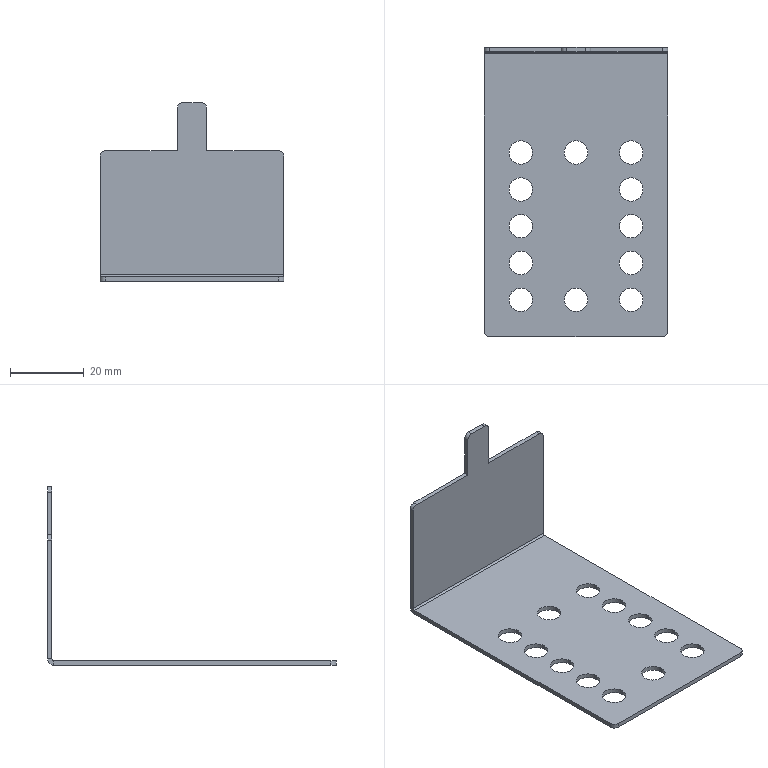Part | SolidWorks | features ICE 2, Extrusion 1, Fillet 1, FlatPattern 1, SheetMetal 1, SolidToSheetMetal 1 | 1 solid | 48 faces | box 50 x 78.5 x 48.5 mm | volume 6398 mm3 | cylinder 32 | plane 16 | commonest cylinder face diameters 6.4 x24 3 x6 1 x1 3.4 x1
STEP:
#1=CARTESIAN_POINT('',(-18.2,10.,0.));
#2=VERTEX_POINT('',#1);
#3=CARTESIAN_POINT('',(-11.8,10.,0.));
#4=VERTEX_POINT('',#3);
#5=CARTESIAN_POINT('',(-15.,10.,0.));
#6=DIRECTION('',(0.,0.,1.));
#7=DIRECTION('',(1.,0.,0.));
#8=AXIS2_PLACEMENT_3D('',#5,#6,#7);
#9=CIRCLE('',#8,3.2);
#10=EDGE_CURVE('',#2,#4,#9,.T.);
#11=ORIENTED_EDGE('',*,*,#10,.F.);
#12=CARTESIAN_POINT('',(-18.2,10.,1.2));
#13=VERTEX_POINT('',#12);
#14=CARTESIAN_POINT('',(-18.2,10.,0.));
#15=DIRECTION('',(0.,0.,1.));
#16=VECTOR('',#15,1000.);
#17=LINE('',#14,#16);
#18=EDGE_CURVE('',#2,#13,#17,.T.);
#19=ORIENTED_EDGE('',*,*,#18,.T.);
#20=CARTESIAN_POINT('',(-11.8,10.,1.2));
#21=VERTEX_POINT('',#20);
#22=CARTESIAN_POINT('',(-15.,10.,1.2));
#23=DIRECTION('',(0.,0.,1.));
#24=DIRECTION('',(1.,0.,0.));
#25=AXIS2_PLACEMENT_3D('',#22,#23,#24);
#26=CIRCLE('',#25,3.2);
#27=EDGE_CURVE('',#13,#21,#26,.T.);
#28=ORIENTED_EDGE('',*,*,#27,.T.);
#29=CARTESIAN_POINT('',(-11.8,10.,0.));
#30=DIRECTION('',(0.,0.,1.));
#31=VECTOR('',#30,1000.);
#32=LINE('',#29,#31);
#33=EDGE_CURVE('',#4,#21,#32,.T.);
#34=ORIENTED_EDGE('',*,*,#33,.F.);
#35=EDGE_LOOP('',(#11,#19,#28,#34));
#36=FACE_OUTER_BOUND('',#35,.T.);
#37=CARTESIAN_POINT('',(-15.,10.,0.));
#38=DIRECTION('',(0.,0.,1.));
#39=DIRECTION('',(1.,0.,0.));
#40=AXIS2_PLACEMENT_3D('',#37,#38,#39);
#41=CYLINDRICAL_SURFACE('',#40,3.2);
#42=ADVANCED_FACE('',(#36),#41,.F.);
#43=CARTESIAN_POINT('',(-18.2,40.,0.));
#44=VERTEX_POINT('',#43);
#45=CARTESIAN_POINT('',(-11.8,40.,0.));
#46=VERTEX_POINT('',#45);
#47=CARTESIAN_POINT('',(-15.,40.,0.));
#48=DIRECTION('',(0.,0.,1.));
#49=DIRECTION('',(1.,0.,0.));
#50=AXIS2_PLACEMENT_3D('',#47,#48,#49);
#51=CIRCLE('',#50,3.2);
#52=EDGE_CURVE('',#44,#46,#51,.T.);
#53=ORIENTED_EDGE('',*,*,#52,.F.);
#54=CARTESIAN_POINT('',(-18.2,40.,1.2));
#55=VERTEX_POINT('',#54);
#56=CARTESIAN_POINT('',(-18.2,40.,0.));
#57=DIRECTION('',(0.,0.,1.));
#58=VECTOR('',#57,1000.);
#59=LINE('',#56,#58);
#60=EDGE_CURVE('',#44,#55,#59,.T.);
#61=ORIENTED_EDGE('',*,*,#60,.T.);
#62=CARTESIAN_POINT('',(-11.8,40.,1.2));
#63=VERTEX_POINT('',#62);
#64=CARTESIAN_POINT('',(-15.,40.,1.2));
#65=DIRECTION('',(0.,0.,1.));
#66=DIRECTION('',(1.,0.,0.));
#67=AXIS2_PLACEMENT_3D('',#64,#65,#66);
#68=CIRCLE('',#67,3.2);
#69=EDGE_CURVE('',#55,#63,#68,.T.);
#70=ORIENTED_EDGE('',*,*,#69,.T.);
#71=CARTESIAN_POINT('',(-11.8,40.,0.));
#72=DIRECTION('',(0.,0.,1.));
#73=VECTOR('',#72,1000.);
#74=LINE('',#71,#73);
#75=EDGE_CURVE('',#46,#63,#74,.T.);
#76=ORIENTED_EDGE('',*,*,#75,.F.);
#77=EDGE_LOOP('',(#53,#61,#70,#76));
#78=FACE_OUTER_BOUND('',#77,.T.);
#79=CARTESIAN_POINT('',(-15.,40.,0.));
#80=DIRECTION('',(0.,0.,1.));
#81=DIRECTION('',(1.,0.,0.));
#82=AXIS2_PLACEMENT_3D('',#79,#80,#81);
#83=CYLINDRICAL_SURFACE('',#82,3.2);
#84=ADVANCED_FACE('',(#78),#83,.F.);
#85=CARTESIAN_POINT('',(-18.2,20.,0.));
#86=VERTEX_POINT('',#85);
#87=CARTESIAN_POINT('',(-11.8,20.,0.));
#88=VERTEX_POINT('',#87);
#89=CARTESIAN_POINT('',(-15.,20.,0.));
#90=DIRECTION('',(0.,0.,1.));
#91=DIRECTION('',(1.,0.,0.));
#92=AXIS2_PLACEMENT_3D('',#89,#90,#91);
#93=CIRCLE('',#92,3.2);
#94=EDGE_CURVE('',#86,#88,#93,.T.);
#95=ORIENTED_EDGE('',*,*,#94,.F.);
#96=CARTESIAN_POINT('',(-18.2,20.,1.2));
#97=VERTEX_POINT('',#96);
#98=CARTESIAN_POINT('',(-18.2,20.,0.));
#99=DIRECTION('',(0.,0.,1.));
#100=VECTOR('',#99,1000.);
#101=LINE('',#98,#100);
#102=EDGE_CURVE('',#86,#97,#101,.T.);
#103=ORIENTED_EDGE('',*,*,#102,.T.);
#104=CARTESIAN_POINT('',(-11.8,20.,1.2));
#105=VERTEX_POINT('',#104);
#106=CARTESIAN_POINT('',(-15.,20.,1.2));
#107=DIRECTION('',(0.,0.,1.));
#108=DIRECTION('',(1.,0.,0.));
#109=AXIS2_PLACEMENT_3D('',#106,#107,#108);
#110=CIRCLE('',#109,3.2);
#111=EDGE_CURVE('',#97,#105,#110,.T.);
#112=ORIENTED_EDGE('',*,*,#111,.T.);
#113=CARTESIAN_POINT('',(-11.8,20.,0.));
#114=DIRECTION('',(0.,0.,1.));
#115=VECTOR('',#114,1000.);
#116=LINE('',#113,#115);
#117=EDGE_CURVE('',#88,#105,#116,.T.);
#118=ORIENTED_EDGE('',*,*,#117,.F.);
#119=EDGE_LOOP('',(#95,#103,#112,#118));
#120=FACE_OUTER_BOUND('',#119,.T.);
#121=CARTESIAN_POINT('',(-15.,20.,0.));
#122=DIRECTION('',(0.,0.,1.));
#123=DIRECTION('',(1.,0.,0.));
#124=AXIS2_PLACEMENT_3D('',#121,#122,#123);
#125=CYLINDRICAL_SURFACE('',#124,3.2);
#126=ADVANCED_FACE('',(#120),#125,.F.);
#127=CARTESIAN_POINT('',(-18.2,30.,0.));
#128=VERTEX_POINT('',#127);
#129=CARTESIAN_POINT('',(-11.8,30.,0.));
#130=VERTEX_POINT('',#129);
#131=CARTESIAN_POINT('',(-15.,30.,0.));
#132=DIRECTION('',(0.,0.,1.));
#133=DIRECTION('',(1.,0.,0.));
#134=AXIS2_PLACEMENT_3D('',#131,#132,#133);
#135=CIRCLE('',#134,3.2);
#136=EDGE_CURVE('',#128,#130,#135,.T.);
#137=ORIENTED_EDGE('',*,*,#136,.F.);
#138=CARTESIAN_POINT('',(-18.2,30.,1.2));
#139=VERTEX_POINT('',#138);
#140=CARTESIAN_POINT('',(-18.2,30.,0.));
#141=DIRECTION('',(0.,0.,1.));
#142=VECTOR('',#141,1000.);
#143=LINE('',#140,#142);
#144=EDGE_CURVE('',#128,#139,#143,.T.);
#145=ORIENTED_EDGE('',*,*,#144,.T.);
#146=CARTESIAN_POINT('',(-11.8,30.,1.2));
#147=VERTEX_POINT('',#146);
#148=CARTESIAN_POINT('',(-15.,30.,1.2));
#149=DIRECTION('',(0.,0.,1.));
#150=DIRECTION('',(1.,0.,0.));
#151=AXIS2_PLACEMENT_3D('',#148,#149,#150);
#152=CIRCLE('',#151,3.2);
#153=EDGE_CURVE('',#139,#147,#152,.T.);
#154=ORIENTED_EDGE('',*,*,#153,.T.);
#155=CARTESIAN_POINT('',(-11.8,30.,0.));
#156=DIRECTION('',(0.,0.,1.));
#157=VECTOR('',#156,1000.);
#158=LINE('',#155,#157);
#159=EDGE_CURVE('',#130,#147,#158,.T.);
#160=ORIENTED_EDGE('',*,*,#159,.F.);
#161=EDGE_LOOP('',(#137,#145,#154,#160));
#162=FACE_OUTER_BOUND('',#161,.T.);
#163=CARTESIAN_POINT('',(-15.,30.,0.));
#164=DIRECTION('',(0.,0.,1.));
#165=DIRECTION('',(1.,0.,0.));
#166=AXIS2_PLACEMENT_3D('',#163,#164,#165);
#167=CYLINDRICAL_SURFACE('',#166,3.2);
#168=ADVANCED_FACE('',(#162),#167,.F.);
#169=CARTESIAN_POINT('',(-18.2,50.,0.));
#170=VERTEX_POINT('',#169);
#171=CARTESIAN_POINT('',(-11.8,50.,0.));
#172=VERTEX_POINT('',#171);
#173=CARTESIAN_POINT('',(-15.,50.,0.));
#174=DIRECTION('',(0.,0.,1.));
#175=DIRECTION('',(1.,0.,0.));
#176=AXIS2_PLACEMENT_3D('',#173,#174,#175);
#177=CIRCLE('',#176,3.2);
#178=EDGE_CURVE('',#170,#172,#177,.T.);
#179=ORIENTED_EDGE('',*,*,#178,.F.);
#180=CARTESIAN_POINT('',(-18.2,50.,1.2));
#181=VERTEX_POINT('',#180);
#182=CARTESIAN_POINT('',(-18.2,50.,0.));
#183=DIRECTION('',(0.,0.,1.));
#184=VECTOR('',#183,1000.);
#185=LINE('',#182,#184);
#186=EDGE_CURVE('',#170,#181,#185,.T.);
#187=ORIENTED_EDGE('',*,*,#186,.T.);
#188=CARTESIAN_POINT('',(-11.8,50.,1.2));
#189=VERTEX_POINT('',#188);
#190=CARTESIAN_POINT('',(-15.,50.,1.2));
#191=DIRECTION('',(0.,0.,1.));
#192=DIRECTION('',(1.,0.,0.));
#193=AXIS2_PLACEMENT_3D('',#190,#191,#192);
#194=CIRCLE('',#193,3.2);
#195=EDGE_CURVE('',#181,#189,#194,.T.);
#196=ORIENTED_EDGE('',*,*,#195,.T.);
#197=CARTESIAN_POINT('',(-11.8,50.,0.));
#198=DIRECTION('',(0.,0.,1.));
#199=VECTOR('',#198,1000.);
#200=LINE('',#197,#199);
#201=EDGE_CURVE('',#172,#189,#200,.T.);
#202=ORIENTED_EDGE('',*,*,#201,.F.);
#203=EDGE_LOOP('',(#179,#187,#196,#202));
#204=FACE_OUTER_BOUND('',#203,.T.);
#205=CARTESIAN_POINT('',(-15.,50.,0.));
#206=DIRECTION('',(0.,0.,1.));
#207=DIRECTION('',(1.,0.,0.));
#208=AXIS2_PLACEMENT_3D('',#205,#206,#207);
#209=CYLINDRICAL_SURFACE('',#208,3.2);
#210=ADVANCED_FACE('',(#204),#209,.F.);
#211=CARTESIAN_POINT('',(11.8,10.,0.));
#212=VERTEX_POINT('',#211);
#213=CARTESIAN_POINT('',(18.2,10.,0.));
#214=VERTEX_POINT('',#213);
#215=CARTESIAN_POINT('',(15.,10.,0.));
#216=DIRECTION('',(0.,0.,1.));
#217=DIRECTION('',(1.,0.,0.));
#218=AXIS2_PLACEMENT_3D('',#215,#216,#217);
#219=CIRCLE('',#218,3.2);
#220=EDGE_CURVE('',#212,#214,#219,.T.);
#221=ORIENTED_EDGE('',*,*,#220,.F.);
#222=CARTESIAN_POINT('',(11.8,10.,1.2));
#223=VERTEX_POINT('',#222);
#224=CARTESIAN_POINT('',(11.8,10.,0.));
#225=DIRECTION('',(0.,0.,1.));
#226=VECTOR('',#225,1000.);
#227=LINE('',#224,#226);
#228=EDGE_CURVE('',#212,#223,#227,.T.);
#229=ORIENTED_EDGE('',*,*,#228,.T.);
#230=CARTESIAN_POINT('',(18.2,10.,1.2));
#231=VERTEX_POINT('',#230);
#232=CARTESIAN_POINT('',(15.,10.,1.2));
#233=DIRECTION('',(0.,0.,1.));
#234=DIRECTION('',(1.,0.,0.));
#235=AXIS2_PLACEMENT_3D('',#232,#233,#234);
#236=CIRCLE('',#235,3.2);
#237=EDGE_CURVE('',#223,#231,#236,.T.);
#238=ORIENTED_EDGE('',*,*,#237,.T.);
#239=CARTESIAN_POINT('',(18.2,10.,0.));
#240=DIRECTION('',(0.,0.,1.));
#241=VECTOR('',#240,1000.);
#242=LINE('',#239,#241);
#243=EDGE_CURVE('',#214,#231,#242,.T.);
#244=ORIENTED_EDGE('',*,*,#243,.F.);
#245=EDGE_LOOP('',(#221,#229,#238,#244));
#246=FACE_OUTER_BOUND('',#245,.T.);
#247=CARTESIAN_POINT('',(15.,10.,0.));
#248=DIRECTION('',(0.,0.,1.));
#249=DIRECTION('',(1.,0.,0.));
#250=AXIS2_PLACEMENT_3D('',#247,#248,#249);
#251=CYLINDRICAL_SURFACE('',#250,3.2);
#252=ADVANCED_FACE('',(#246),#251,.F.);
#253=CARTESIAN_POINT('',(11.8,40.,0.));
#254=VERTEX_POINT('',#253);
#255=CARTESIAN_POINT('',(18.2,40.,0.));
#256=VERTEX_POINT('',#255);
#257=CARTESIAN_POINT('',(15.,40.,0.));
#258=DIRECTION('',(0.,0.,1.));
#259=DIRECTION('',(1.,0.,0.));
#260=AXIS2_PLACEMENT_3D('',#257,#258,#259);
#261=CIRCLE('',#260,3.2);
#262=EDGE_CURVE('',#254,#256,#261,.T.);
#263=ORIENTED_EDGE('',*,*,#262,.F.);
#264=CARTESIAN_POINT('',(11.8,40.,1.2));
#265=VERTEX_POINT('',#264);
#266=CARTESIAN_POINT('',(11.8,40.,0.));
#267=DIRECTION('',(0.,0.,1.));
#268=VECTOR('',#267,1000.);
#269=LINE('',#266,#268);
#270=EDGE_CURVE('',#254,#265,#269,.T.);
#271=ORIENTED_EDGE('',*,*,#270,.T.);
#272=CARTESIAN_POINT('',(18.2,40.,1.2));
#273=VERTEX_POINT('',#272);
#274=CARTESIAN_POINT('',(15.,40.,1.2));
#275=DIRECTION('',(0.,0.,1.));
#276=DIRECTION('',(1.,0.,0.));
#277=AXIS2_PLACEMENT_3D('',#274,#275,#276);
#278=CIRCLE('',#277,3.2);
#279=EDGE_CURVE('',#265,#273,#278,.T.);
#280=ORIENTED_EDGE('',*,*,#279,.T.);
#281=CARTESIAN_POINT('',(18.2,40.,0.));
#282=DIRECTION('',(0.,0.,1.));
#283=VECTOR('',#282,1000.);
#284=LINE('',#281,#283);
#285=EDGE_CURVE('',#256,#273,#284,.T.);
#286=ORIENTED_EDGE('',*,*,#285,.F.);
#287=EDGE_LOOP('',(#263,#271,#280,#286));
#288=FACE_OUTER_BOUND('',#287,.T.);
#289=CARTESIAN_POINT('',(15.,40.,0.));
#290=DIRECTION('',(0.,0.,1.));
#291=DIRECTION('',(1.,0.,0.));
#292=AXIS2_PLACEMENT_3D('',#289,#290,#291);
#293=CYLINDRICAL_SURFACE('',#292,3.2);
#294=ADVANCED_FACE('',(#288),#293,.F.);
#295=CARTESIAN_POINT('',(11.8,20.,0.));
#296=VERTEX_POINT('',#295);
#297=CARTESIAN_POINT('',(18.2,20.,0.));
#298=VERTEX_POINT('',#297);
#299=CARTESIAN_POINT('',(15.,20.,0.));
#300=DIRECTION('',(0.,0.,1.));
#301=DIRECTION('',(1.,0.,0.));
#302=AXIS2_PLACEMENT_3D('',#299,#300,#301);
#303=CIRCLE('',#302,3.2);
#304=EDGE_CURVE('',#296,#298,#303,.T.);
#305=ORIENTED_EDGE('',*,*,#304,.F.);
#306=CARTESIAN_POINT('',(11.8,20.,1.2));
#307=VERTEX_POINT('',#306);
#308=CARTESIAN_POINT('',(11.8,20.,0.));
#309=DIRECTION('',(0.,0.,1.));
#310=VECTOR('',#309,1000.);
#311=LINE('',#308,#310);
#312=EDGE_CURVE('',#296,#307,#311,.T.);
#313=ORIENTED_EDGE('',*,*,#312,.T.);
#314=CARTESIAN_POINT('',(18.2,20.,1.2));
#315=VERTEX_POINT('',#314);
#316=CARTESIAN_POINT('',(15.,20.,1.2));
#317=DIRECTION('',(0.,0.,1.));
#318=DIRECTION('',(1.,0.,0.));
#319=AXIS2_PLACEMENT_3D('',#316,#317,#318);
#320=CIRCLE('',#319,3.2);
#321=EDGE_CURVE('',#307,#315,#320,.T.);
#322=ORIENTED_EDGE('',*,*,#321,.T.);
#323=CARTESIAN_POINT('',(18.2,20.,0.));
#324=DIRECTION('',(0.,0.,1.));
#325=VECTOR('',#324,1000.);
#326=LINE('',#323,#325);
#327=EDGE_CURVE('',#298,#315,#326,.T.);
#328=ORIENTED_EDGE('',*,*,#327,.F.);
#329=EDGE_LOOP('',(#305,#313,#322,#328));
#330=FACE_OUTER_BOUND('',#329,.T.);
#331=CARTESIAN_POINT('',(15.,20.,0.));
#332=DIRECTION('',(0.,0.,1.));
#333=DIRECTION('',(1.,0.,0.));
#334=AXIS2_PLACEMENT_3D('',#331,#332,#333);
#335=CYLINDRICAL_SURFACE('',#334,3.2);
#336=ADVANCED_FACE('',(#330),#335,.F.);
#337=CARTESIAN_POINT('',(11.8,30.,0.));
#338=VERTEX_POINT('',#337);
#339=CARTESIAN_POINT('',(18.2,30.,0.));
#340=VERTEX_POINT('',#339);
#341=CARTESIAN_POINT('',(15.,30.,0.));
#342=DIRECTION('',(0.,0.,1.));
#343=DIRECTION('',(1.,0.,0.));
#344=AXIS2_PLACEMENT_3D('',#341,#342,#343);
#345=CIRCLE('',#344,3.2);
#346=EDGE_CURVE('',#338,#340,#345,.T.);
#347=ORIENTED_EDGE('',*,*,#346,.F.);
#348=CARTESIAN_POINT('',(11.8,30.,1.2));
#349=VERTEX_POINT('',#348);
#350=CARTESIAN_POINT('',(11.8,30.,0.));
#351=DIRECTION('',(0.,0.,1.));
#352=VECTOR('',#351,1000.);
#353=LINE('',#350,#352);
#354=EDGE_CURVE('',#338,#349,#353,.T.);
#355=ORIENTED_EDGE('',*,*,#354,.T.);
#356=CARTESIAN_POINT('',(18.2,30.,1.2));
#357=VERTEX_POINT('',#356);
#358=CARTESIAN_POINT('',(15.,30.,1.2));
#359=DIRECTION('',(0.,0.,1.));
#360=DIRECTION('',(1.,0.,0.));
#361=AXIS2_PLACEMENT_3D('',#358,#359,#360);
#362=CIRCLE('',#361,3.2);
#363=EDGE_CURVE('',#349,#357,#362,.T.);
#364=ORIENTED_EDGE('',*,*,#363,.T.);
#365=CARTESIAN_POINT('',(18.2,30.,0.));
#366=DIRECTION('',(0.,0.,1.));
#367=VECTOR('',#366,1000.);
#368=LINE('',#365,#367);
#369=EDGE_CURVE('',#340,#357,#368,.T.);
#370=ORIENTED_EDGE('',*,*,#369,.F.);
#371=EDGE_LOOP('',(#347,#355,#364,#370));
#372=FACE_OUTER_BOUND('',#371,.T.);
#373=CARTESIAN_POINT('',(15.,30.,0.));
#374=DIRECTION('',(0.,0.,1.));
#375=DIRECTION('',(1.,0.,0.));
#376=AXIS2_PLACEMENT_3D('',#373,#374,#375);
#377=CYLINDRICAL_SURFACE('',#376,3.2);
#378=ADVANCED_FACE('',(#372),#377,.F.);
#379=CARTESIAN_POINT('',(11.8,50.,0.));
#380=VERTEX_POINT('',#379);
#381=CARTESIAN_POINT('',(18.2,50.,0.));
#382=VERTEX_POINT('',#381);
#383=CARTESIAN_POINT('',(15.,50.,0.));
#384=DIRECTION('',(0.,0.,1.));
#385=DIRECTION('',(1.,0.,0.));
#386=AXIS2_PLACEMENT_3D('',#383,#384,#385);
#387=CIRCLE('',#386,3.2);
#388=EDGE_CURVE('',#380,#382,#387,.T.);
#389=ORIENTED_EDGE('',*,*,#388,.F.);
#390=CARTESIAN_POINT('',(11.8,50.,1.2));
#391=VERTEX_POINT('',#390);
#392=CARTESIAN_POINT('',(11.8,50.,0.));
#393=DIRECTION('',(0.,0.,1.));
#394=VECTOR('',#393,1000.);
#395=LINE('',#392,#394);
#396=EDGE_CURVE('',#380,#391,#395,.T.);
#397=ORIENTED_EDGE('',*,*,#396,.T.);
#398=CARTESIAN_POINT('',(18.2,50.,1.2));
#399=VERTEX_POINT('',#398);
#400=CARTESIAN_POINT('',(15.,50.,1.2));
#401=DIRECTION('',(0.,0.,1.));
#402=DIRECTION('',(1.,0.,0.));
#403=AXIS2_PLACEMENT_3D('',#400,#401,#402);
#404=CIRCLE('',#403,3.2);
#405=EDGE_CURVE('',#391,#399,#404,.T.);
#406=ORIENTED_EDGE('',*,*,#405,.T.);
#407=CARTESIAN_POINT('',(18.2,50.,0.));
#408=DIRECTION('',(0.,0.,1.));
#409=VECTOR('',#408,1000.);
#410=LINE('',#407,#409);
#411=EDGE_CURVE('',#382,#399,#410,.T.);
#412=ORIENTED_EDGE('',*,*,#411,.F.);
#413=EDGE_LOOP('',(#389,#397,#406,#412));
#414=FACE_OUTER_BOUND('',#413,.T.);
#415=CARTESIAN_POINT('',(15.,50.,0.));
#416=DIRECTION('',(0.,0.,1.));
#417=DIRECTION('',(1.,0.,0.));
#418=AXIS2_PLACEMENT_3D('',#415,#416,#417);
#419=CYLINDRICAL_SURFACE('',#418,3.2);
#420=ADVANCED_FACE('',(#414),#419,.F.);
#421=CARTESIAN_POINT('',(-3.2,50.,0.));
#422=VERTEX_POINT('',#421);
#423=CARTESIAN_POINT('',(3.2,50.,0.));
#424=VERTEX_POINT('',#423);
#425=CARTESIAN_POINT('',(0.,50.,0.));
#426=DIRECTION('',(0.,0.,1.));
#427=DIRECTION('',(1.,0.,0.));
#428=AXIS2_PLACEMENT_3D('',#425,#426,#427);
#429=CIRCLE('',#428,3.2);
#430=EDGE_CURVE('',#422,#424,#429,.T.);
#431=ORIENTED_EDGE('',*,*,#430,.F.);
#432=CARTESIAN_POINT('',(-3.2,50.,1.2));
#433=VERTEX_POINT('',#432);
#434=CARTESIAN_POINT('',(-3.2,50.,0.));
#435=DIRECTION('',(0.,0.,1.));
#436=VECTOR('',#435,1000.);
#437=LINE('',#434,#436);
#438=EDGE_CURVE('',#422,#433,#437,.T.);
#439=ORIENTED_EDGE('',*,*,#438,.T.);
#440=CARTESIAN_POINT('',(3.2,50.,1.2));
#441=VERTEX_POINT('',#440);
#442=CARTESIAN_POINT('',(0.,50.,1.2));
#443=DIRECTION('',(0.,0.,1.));
#444=DIRECTION('',(1.,0.,0.));
#445=AXIS2_PLACEMENT_3D('',#442,#443,#444);
#446=CIRCLE('',#445,3.2);
#447=EDGE_CURVE('',#433,#441,#446,.T.);
#448=ORIENTED_EDGE('',*,*,#447,.T.);
#449=CARTESIAN_POINT('',(3.2,50.,0.));
#450=DIRECTION('',(0.,0.,1.));
#451=VECTOR('',#450,1000.);
#452=LINE('',#449,#451);
#453=EDGE_CURVE('',#424,#441,#452,.T.);
#454=ORIENTED_EDGE('',*,*,#453,.F.);
#455=EDGE_LOOP('',(#431,#439,#448,#454));
#456=FACE_OUTER_BOUND('',#455,.T.);
#457=CARTESIAN_POINT('',(0.,50.,0.));
#458=DIRECTION('',(0.,0.,1.));
#459=DIRECTION('',(1.,0.,0.));
#460=AXIS2_PLACEMENT_3D('',#457,#458,#459);
#461=CYLINDRICAL_SURFACE('',#460,3.2);
#462=ADVANCED_FACE('',(#456),#461,.F.);
#463=CARTESIAN_POINT('',(-3.2,10.,0.));
#464=VERTEX_POINT('',#463);
#465=CARTESIAN_POINT('',(3.2,10.,0.));
#466=VERTEX_POINT('',#465);
#467=CARTESIAN_POINT('',(0.,10.,0.));
#468=DIRECTION('',(0.,0.,1.));
#469=DIRECTION('',(1.,0.,0.));
#470=AXIS2_PLACEMENT_3D('',#467,#468,#469);
#471=CIRCLE('',#470,3.2);
#472=EDGE_CURVE('',#464,#466,#471,.T.);
#473=ORIENTED_EDGE('',*,*,#472,.F.);
#474=CARTESIAN_POINT('',(-3.2,10.,1.2));
#475=VERTEX_POINT('',#474);
#476=CARTESIAN_POINT('',(-3.2,10.,0.));
#477=DIRECTION('',(0.,0.,1.));
#478=VECTOR('',#477,1000.);
#479=LINE('',#476,#478);
#480=EDGE_CURVE('',#464,#475,#479,.T.);
#481=ORIENTED_EDGE('',*,*,#480,.T.);
#482=CARTESIAN_POINT('',(3.2,10.,1.2));
#483=VERTEX_POINT('',#482);
#484=CARTESIAN_POINT('',(0.,10.,1.2));
#485=DIRECTION('',(0.,0.,1.));
#486=DIRECTION('',(1.,0.,0.));
#487=AXIS2_PLACEMENT_3D('',#484,#485,#486);
#488=CIRCLE('',#487,3.2);
#489=EDGE_CURVE('',#475,#483,#488,.T.);
#490=ORIENTED_EDGE('',*,*,#489,.T.);
#491=CARTESIAN_POINT('',(3.2,10.,0.));
#492=DIRECTION('',(0.,0.,1.));
#493=VECTOR('',#492,1000.);
#494=LINE('',#491,#493);
#495=EDGE_CURVE('',#466,#483,#494,.T.);
#496=ORIENTED_EDGE('',*,*,#495,.F.);
#497=EDGE_LOOP('',(#473,#481,#490,#496));
#498=FACE_OUTER_BOUND('',#497,.T.);
#499=CARTESIAN_POINT('',(0.,10.,0.));
#500=DIRECTION('',(0.,0.,1.));
#501=DIRECTION('',(1.,0.,0.));
#502=AXIS2_PLACEMENT_3D('',#499,#500,#501);
#503=CYLINDRICAL_SURFACE('',#502,3.2);
#504=ADVANCED_FACE('',(#498),#503,.F.);
#505=CARTESIAN_POINT('',(25.,76.8,1.2));
#506=VERTEX_POINT('',#505);
#507=CARTESIAN_POINT('',(25.,76.8,0.));
#508=VERTEX_POINT('',#507);
#509=CARTESIAN_POINT('',(25.,76.8,0.));
#510=DIRECTION('',(0.,0.,-1.));
#511=VECTOR('',#510,1000.);
#512=LINE('',#509,#511);
#513=EDGE_CURVE('',#506,#508,#512,.T.);
#514=ORIENTED_EDGE('',*,*,#513,.F.);
#515=CARTESIAN_POINT('',(25.,1.5,1.2));
#516=VERTEX_POINT('',#515);
#517=CARTESIAN_POINT('',(25.,0.,1.2));
#518=DIRECTION('',(0.,1.,0.));
#519=VECTOR('',#518,1000.);
#520=LINE('',#517,#519);
#521=EDGE_CURVE('',#516,#506,#520,.T.);
#522=ORIENTED_EDGE('',*,*,#521,.F.);
#523=CARTESIAN_POINT('',(25.,1.5,0.));
#524=VERTEX_POINT('',#523);
#525=CARTESIAN_POINT('',(25.,1.5,0.));
#526=DIRECTION('',(0.,0.,-1.));
#527=VECTOR('',#526,1000.);
#528=LINE('',#525,#527);
#529=EDGE_CURVE('',#516,#524,#528,.T.);
#530=ORIENTED_EDGE('',*,*,#529,.T.);
#531=CARTESIAN_POINT('',(25.,0.,0.));
#532=DIRECTION('',(0.,1.,0.));
#533=VECTOR('',#532,1000.);
#534=LINE('',#531,#533);
#535=EDGE_CURVE('',#524,#508,#534,.T.);
#536=ORIENTED_EDGE('',*,*,#535,.T.);
#537=EDGE_LOOP('',(#514,#522,#530,#536));
#538=FACE_OUTER_BOUND('',#537,.T.);
#539=CARTESIAN_POINT('',(25.,0.,0.));
#540=DIRECTION('',(1.,0.,0.));
#541=DIRECTION('',(0.,1.,0.));
#542=AXIS2_PLACEMENT_3D('',#539,#540,#541);
#543=PLANE('',#542);
#544=ADVANCED_FACE('',(#538),#543,.T.);
#545=ORIENTED_EDGE('',*,*,#529,.F.);
#546=CARTESIAN_POINT('',(23.5,0.,1.2));
#547=VERTEX_POINT('',#546);
#548=CARTESIAN_POINT('',(23.5,1.5,1.2));
#549=DIRECTION('',(0.,0.,-1.));
#550=DIRECTION('',(1.,0.,0.));
#551=AXIS2_PLACEMENT_3D('',#548,#549,#550);
#552=CIRCLE('',#551,1.5);
#553=EDGE_CURVE('',#516,#547,#552,.T.);
#554=ORIENTED_EDGE('',*,*,#553,.T.);
#555=CARTESIAN_POINT('',(23.5,0.,0.));
#556=VERTEX_POINT('',#555);
#557=CARTESIAN_POINT('',(23.5,0.,0.));
#558=DIRECTION('',(0.,0.,-1.));
#559=VECTOR('',#558,1000.);
#560=LINE('',#557,#559);
#561=EDGE_CURVE('',#547,#556,#560,.T.);
#562=ORIENTED_EDGE('',*,*,#561,.T.);
#563=CARTESIAN_POINT('',(23.5,1.5,0.));
#564=DIRECTION('',(0.,0.,-1.));
#565=DIRECTION('',(1.,0.,0.));
#566=AXIS2_PLACEMENT_3D('',#563,#564,#565);
#567=CIRCLE('',#566,1.5);
#568=EDGE_CURVE('',#524,#556,#567,.T.);
#569=ORIENTED_EDGE('',*,*,#568,.F.);
#570=EDGE_LOOP('',(#545,#554,#562,#569));
#571=FACE_OUTER_BOUND('',#570,.T.);
#572=CARTESIAN_POINT('',(23.5,1.5,0.));
#573=DIRECTION('',(0.,0.,1.));
#574=DIRECTION('',(1.,0.,0.));
#575=AXIS2_PLACEMENT_3D('',#572,#573,#574);
#576=CYLINDRICAL_SURFACE('',#575,1.5);
#577=ADVANCED_FACE('',(#571),#576,.T.);
#578=ORIENTED_EDGE('',*,*,#561,.F.);
#579=CARTESIAN_POINT('',(-23.5,0.,1.2));
#580=VERTEX_POINT('',#579);
#581=CARTESIAN_POINT('',(0.,0.,1.2));
#582=DIRECTION('',(1.,0.,0.));
#583=VECTOR('',#582,1000.);
#584=LINE('',#581,#583);
#585=EDGE_CURVE('',#580,#547,#584,.T.);
#586=ORIENTED_EDGE('',*,*,#585,.F.);
#587=CARTESIAN_POINT('',(-23.5,0.,0.));
#588=VERTEX_POINT('',#587);
#589=CARTESIAN_POINT('',(-23.5,0.,0.));
#590=DIRECTION('',(0.,0.,-1.));
#591=VECTOR('',#590,1000.);
#592=LINE('',#589,#591);
#593=EDGE_CURVE('',#580,#588,#592,.T.);
#594=ORIENTED_EDGE('',*,*,#593,.T.);
#595=CARTESIAN_POINT('',(0.,0.,0.));
#596=DIRECTION('',(1.,0.,0.));
#597=VECTOR('',#596,1000.);
#598=LINE('',#595,#597);
#599=EDGE_CURVE('',#588,#556,#598,.T.);
#600=ORIENTED_EDGE('',*,*,#599,.T.);
#601=EDGE_LOOP('',(#578,#586,#594,#600));
#602=FACE_OUTER_BOUND('',#601,.T.);
#603=CARTESIAN_POINT('',(0.,0.,0.));
#604=DIRECTION('',(0.,-1.,0.));
#605=DIRECTION('',(1.,0.,0.));
#606=AXIS2_PLACEMENT_3D('',#603,#604,#605);
#607=PLANE('',#606);
#608=ADVANCED_FACE('',(#602),#607,.T.);
#609=ORIENTED_EDGE('',*,*,#593,.F.);
#610=CARTESIAN_POINT('',(-25.,1.5,1.2));
#611=VERTEX_POINT('',#610);
#612=CARTESIAN_POINT('',(-23.5,1.5,1.2));
#613=DIRECTION('',(0.,0.,-1.));
#614=DIRECTION('',(1.,0.,0.));
#615=AXIS2_PLACEMENT_3D('',#612,#613,#614);
#616=CIRCLE('',#615,1.5);
#617=EDGE_CURVE('',#580,#611,#616,.T.);
#618=ORIENTED_EDGE('',*,*,#617,.T.);
#619=CARTESIAN_POINT('',(-25.,1.5,0.));
#620=VERTEX_POINT('',#619);
#621=CARTESIAN_POINT('',(-25.,1.5,0.));
#622=DIRECTION('',(0.,0.,-1.));
#623=VECTOR('',#622,1000.);
#624=LINE('',#621,#623);
#625=EDGE_CURVE('',#611,#620,#624,.T.);
#626=ORIENTED_EDGE('',*,*,#625,.T.);
#627=CARTESIAN_POINT('',(-23.5,1.5,0.));
#628=DIRECTION('',(0.,0.,-1.));
#629=DIRECTION('',(1.,0.,0.));
#630=AXIS2_PLACEMENT_3D('',#627,#628,#629);
#631=CIRCLE('',#630,1.5);
#632=EDGE_CURVE('',#588,#620,#631,.T.);
#633=ORIENTED_EDGE('',*,*,#632,.F.);
#634=EDGE_LOOP('',(#609,#618,#626,#633));
#635=FACE_OUTER_BOUND('',#634,.T.);
#636=CARTESIAN_POINT('',(-23.5,1.5,0.));
#637=DIRECTION('',(0.,0.,1.));
#638=DIRECTION('',(1.,0.,0.));
#639=AXIS2_PLACEMENT_3D('',#636,#637,#638);
#640=CYLINDRICAL_SURFACE('',#639,1.5);
#641=ADVANCED_FACE('',(#635),#640,.T.);
#642=ORIENTED_EDGE('',*,*,#625,.F.);
#643=CARTESIAN_POINT('',(-25.,76.8,1.2));
#644=VERTEX_POINT('',#643);
#645=CARTESIAN_POINT('',(-25.,0.,1.2));
#646=DIRECTION('',(0.,1.,0.));
#647=VECTOR('',#646,1000.);
#648=LINE('',#645,#647);
#649=EDGE_CURVE('',#611,#644,#648,.T.);
#650=ORIENTED_EDGE('',*,*,#649,.T.);
#651=CARTESIAN_POINT('',(-25.,76.8,0.));
#652=VERTEX_POINT('',#651);
#653=CARTESIAN_POINT('',(-25.,76.8,0.));
#654=DIRECTION('',(0.,0.,-1.));
#655=VECTOR('',#654,1000.);
#656=LINE('',#653,#655);
#657=EDGE_CURVE('',#644,#652,#656,.T.);
#658=ORIENTED_EDGE('',*,*,#657,.T.);
#659=CARTESIAN_POINT('',(-25.,0.,0.));
#660=DIRECTION('',(0.,1.,0.));
#661=VECTOR('',#660,1000.);
#662=LINE('',#659,#661);
#663=EDGE_CURVE('',#620,#652,#662,.T.);
#664=ORIENTED_EDGE('',*,*,#663,.F.);
#665=EDGE_LOOP('',(#642,#650,#658,#664));
#666=FACE_OUTER_BOUND('',#665,.T.);
#667=CARTESIAN_POINT('',(-25.,0.,0.));
#668=DIRECTION('',(1.,0.,0.));
#669=DIRECTION('',(0.,1.,0.));
#670=AXIS2_PLACEMENT_3D('',#667,#668,#669);
#671=PLANE('',#670);
#672=ADVANCED_FACE('',(#666),#671,.F.);
#673=ORIENTED_EDGE('',*,*,#657,.F.);
#674=CARTESIAN_POINT('',(-25.,77.3,1.7));
#675=VERTEX_POINT('',#674);
#676=CARTESIAN_POINT('',(-25.,76.8,1.7));
#677=DIRECTION('',(1.,0.,0.));
#678=DIRECTION('',(0.,0.,1.));
#679=AXIS2_PLACEMENT_3D('',#676,#677,#678);
#680=CIRCLE('',#679,0.5);
#681=EDGE_CURVE('',#644,#675,#680,.T.);
#682=ORIENTED_EDGE('',*,*,#681,.T.);
#683=CARTESIAN_POINT('',(-25.,78.5,1.7));
#684=VERTEX_POINT('',#683);
#685=CARTESIAN_POINT('',(-25.,78.5,1.7));
#686=DIRECTION('',(0.,1.,0.));
#687=VECTOR('',#686,1000.);
#688=LINE('',#685,#687);
#689=EDGE_CURVE('',#675,#684,#688,.T.);
#690=ORIENTED_EDGE('',*,*,#689,.T.);
#691=CARTESIAN_POINT('',(-25.,76.8,1.7));
#692=DIRECTION('',(1.,0.,0.));
#693=DIRECTION('',(0.,0.,-1.));
#694=AXIS2_PLACEMENT_3D('',#691,#692,#693);
#695=CIRCLE('',#694,1.7);
#696=EDGE_CURVE('',#652,#684,#695,.T.);
#697=ORIENTED_EDGE('',*,*,#696,.F.);
#698=EDGE_LOOP('',(#673,#682,#690,#697));
#699=FACE_OUTER_BOUND('',#698,.T.);
#700=CARTESIAN_POINT('',(-25.,76.8,1.7));
#701=DIRECTION('',(-1.,0.,0.));
#702=DIRECTION('',(0.,0.,1.));
#703=AXIS2_PLACEMENT_3D('',#700,#701,#702);
#704=PLANE('',#703);
#705=ADVANCED_FACE('',(#699),#704,.T.);
#706=ORIENTED_EDGE('',*,*,#689,.F.);
#707=CARTESIAN_POINT('',(-25.,77.3,34.));
#708=VERTEX_POINT('',#707);
#709=CARTESIAN_POINT('',(-25.,77.3,1.2));
#710=DIRECTION('',(0.,0.,-1.));
#711=VECTOR('',#710,1000.);
#712=LINE('',#709,#711);
#713=EDGE_CURVE('',#708,#675,#712,.T.);
#714=ORIENTED_EDGE('',*,*,#713,.F.);
#715=CARTESIAN_POINT('',(-25.,78.5,34.));
#716=VERTEX_POINT('',#715);
#717=CARTESIAN_POINT('',(-25.,78.5,34.));
#718=DIRECTION('',(0.,1.,0.));
#719=VECTOR('',#718,1000.);
#720=LINE('',#717,#719);
#721=EDGE_CURVE('',#708,#716,#720,.T.);
#722=ORIENTED_EDGE('',*,*,#721,.T.);
#723=CARTESIAN_POINT('',(-25.,78.5,1.2));
#724=DIRECTION('',(0.,0.,-1.));
#725=VECTOR('',#724,1000.);
#726=LINE('',#723,#725);
#727=EDGE_CURVE('',#716,#684,#726,.T.);
#728=ORIENTED_EDGE('',*,*,#727,.T.);
#729=EDGE_LOOP('',(#706,#714,#722,#728));
#730=FACE_OUTER_BOUND('',#729,.T.);
#731=CARTESIAN_POINT('',(-25.,78.5,1.2));
#732=DIRECTION('',(1.,0.,0.));
#733=DIRECTION('',(0.,0.,-1.));
#734=AXIS2_PLACEMENT_3D('',#731,#732,#733);
#735=PLANE('',#734);
#736=ADVANCED_FACE('',(#730),#735,.F.);
#737=ORIENTED_EDGE('',*,*,#721,.F.);
#738=CARTESIAN_POINT('',(-23.5,77.3,35.5));
#739=VERTEX_POINT('',#738);
#740=CARTESIAN_POINT('',(-23.5,77.3,34.));
#741=DIRECTION('',(0.,1.,0.));
#742=DIRECTION('',(0.,0.,1.));
#743=AXIS2_PLACEMENT_3D('',#740,#741,#742);
#744=CIRCLE('',#743,1.5);
#745=EDGE_CURVE('',#708,#739,#744,.T.);
#746=ORIENTED_EDGE('',*,*,#745,.T.);
#747=CARTESIAN_POINT('',(-23.5,78.5,35.5));
#748=VERTEX_POINT('',#747);
#749=CARTESIAN_POINT('',(-23.5,78.5,35.5));
#750=DIRECTION('',(0.,1.,0.));
#751=VECTOR('',#750,1000.);
#752=LINE('',#749,#751);
#753=EDGE_CURVE('',#739,#748,#752,.T.);
#754=ORIENTED_EDGE('',*,*,#753,.T.);
#755=CARTESIAN_POINT('',(-23.5,78.5,34.));
#756=DIRECTION('',(0.,1.,0.));
#757=DIRECTION('',(0.,0.,1.));
#758=AXIS2_PLACEMENT_3D('',#755,#756,#757);
#759=CIRCLE('',#758,1.5);
#760=EDGE_CURVE('',#716,#748,#759,.T.);
#761=ORIENTED_EDGE('',*,*,#760,.F.);
#762=EDGE_LOOP('',(#737,#746,#754,#761));
#763=FACE_OUTER_BOUND('',#762,.T.);
#764=CARTESIAN_POINT('',(-23.5,78.5,34.));
#765=DIRECTION('',(0.,1.,0.));
#766=DIRECTION('',(0.,0.,1.));
#767=AXIS2_PLACEMENT_3D('',#764,#765,#766);
#768=CYLINDRICAL_SURFACE('',#767,1.5);
#769=ADVANCED_FACE('',(#763),#768,.T.);
#770=ORIENTED_EDGE('',*,*,#753,.F.);
#771=CARTESIAN_POINT('',(-4.,77.3,35.5));
#772=VERTEX_POINT('',#771);
#773=CARTESIAN_POINT('',(0.,77.3,35.5));
#774=DIRECTION('',(-1.,0.,0.));
#775=VECTOR('',#774,1000.);
#776=LINE('',#773,#775);
#777=EDGE_CURVE('',#772,#739,#776,.T.);
#778=ORIENTED_EDGE('',*,*,#777,.F.);
#779=CARTESIAN_POINT('',(-4.,78.5,35.5));
#780=VERTEX_POINT('',#779);
#781=CARTESIAN_POINT('',(-4.,78.5,35.5));
#782=DIRECTION('',(0.,1.,0.));
#783=VECTOR('',#782,1000.);
#784=LINE('',#781,#783);
#785=EDGE_CURVE('',#772,#780,#784,.T.);
#786=ORIENTED_EDGE('',*,*,#785,.T.);
#787=CARTESIAN_POINT('',(-25.,78.5,35.5));
#788=DIRECTION('',(-1.,0.,0.));
#789=VECTOR('',#788,1000.);
#790=LINE('',#787,#789);
#791=EDGE_CURVE('',#780,#748,#790,.T.);
#792=ORIENTED_EDGE('',*,*,#791,.T.);
#793=EDGE_LOOP('',(#770,#778,#786,#792));
#794=FACE_OUTER_BOUND('',#793,.T.);
#795=CARTESIAN_POINT('',(-25.,78.5,35.5));
#796=DIRECTION('',(0.,0.,-1.));
#797=DIRECTION('',(-1.,0.,0.));
#798=AXIS2_PLACEMENT_3D('',#795,#796,#797);
#799=PLANE('',#798);
#800=ADVANCED_FACE('',(#794),#799,.F.);
#801=ORIENTED_EDGE('',*,*,#785,.F.);
#802=CARTESIAN_POINT('',(-4.,77.3,47.));
#803=VERTEX_POINT('',#802);
#804=CARTESIAN_POINT('',(-4.,77.3,1.2));
#805=DIRECTION('',(0.,0.,-1.));
#806=VECTOR('',#805,1000.);
#807=LINE('',#804,#806);
#808=EDGE_CURVE('',#803,#772,#807,.T.);
#809=ORIENTED_EDGE('',*,*,#808,.F.);
#810=CARTESIAN_POINT('',(-4.,78.5,47.));
#811=VERTEX_POINT('',#810);
#812=CARTESIAN_POINT('',(-4.,78.5,47.));
#813=DIRECTION('',(0.,1.,0.));
#814=VECTOR('',#813,1000.);
#815=LINE('',#812,#814);
#816=EDGE_CURVE('',#803,#811,#815,.T.);
#817=ORIENTED_EDGE('',*,*,#816,.T.);
#818=CARTESIAN_POINT('',(-4.,78.5,48.5));
#819=DIRECTION('',(0.,0.,-1.));
#820=VECTOR('',#819,1000.);
#821=LINE('',#818,#820);
#822=EDGE_CURVE('',#811,#780,#821,.T.);
#823=ORIENTED_EDGE('',*,*,#822,.T.);
#824=EDGE_LOOP('',(#801,#809,#817,#823));
#825=FACE_OUTER_BOUND('',#824,.T.);
#826=CARTESIAN_POINT('',(-4.,78.5,48.5));
#827=DIRECTION('',(1.,0.,0.));
#828=DIRECTION('',(0.,0.,-1.));
#829=AXIS2_PLACEMENT_3D('',#826,#827,#828);
#830=PLANE('',#829);
#831=ADVANCED_FACE('',(#825),#830,.F.);
#832=ORIENTED_EDGE('',*,*,#816,.F.);
#833=CARTESIAN_POINT('',(-2.5,77.3,48.5));
#834=VERTEX_POINT('',#833);
#835=CARTESIAN_POINT('',(-2.5,77.3,47.));
#836=DIRECTION('',(0.,1.,0.));
#837=DIRECTION('',(0.,0.,1.));
#838=AXIS2_PLACEMENT_3D('',#835,#836,#837);
#839=CIRCLE('',#838,1.5);
#840=EDGE_CURVE('',#803,#834,#839,.T.);
#841=ORIENTED_EDGE('',*,*,#840,.T.);
#842=CARTESIAN_POINT('',(-2.5,78.5,48.5));
#843=VERTEX_POINT('',#842);
#844=CARTESIAN_POINT('',(-2.5,78.5,48.5));
#845=DIRECTION('',(0.,1.,0.));
#846=VECTOR('',#845,1000.);
#847=LINE('',#844,#846);
#848=EDGE_CURVE('',#834,#843,#847,.T.);
#849=ORIENTED_EDGE('',*,*,#848,.T.);
#850=CARTESIAN_POINT('',(-2.5,78.5,47.));
#851=DIRECTION('',(0.,1.,0.));
#852=DIRECTION('',(0.,0.,1.));
#853=AXIS2_PLACEMENT_3D('',#850,#851,#852);
#854=CIRCLE('',#853,1.5);
#855=EDGE_CURVE('',#811,#843,#854,.T.);
#856=ORIENTED_EDGE('',*,*,#855,.F.);
#857=EDGE_LOOP('',(#832,#841,#849,#856));
#858=FACE_OUTER_BOUND('',#857,.T.);
#859=CARTESIAN_POINT('',(-2.5,78.5,47.));
#860=DIRECTION('',(0.,1.,0.));
#861=DIRECTION('',(0.,0.,1.));
#862=AXIS2_PLACEMENT_3D('',#859,#860,#861);
#863=CYLINDRICAL_SURFACE('',#862,1.5);
#864=ADVANCED_FACE('',(#858),#863,.T.);
#865=ORIENTED_EDGE('',*,*,#848,.F.);
#866=CARTESIAN_POINT('',(2.5,77.3,48.5));
#867=VERTEX_POINT('',#866);
#868=CARTESIAN_POINT('',(0.,77.3,48.5));
#869=DIRECTION('',(-1.,0.,0.));
#870=VECTOR('',#869,1000.);
#871=LINE('',#868,#870);
#872=EDGE_CURVE('',#867,#834,#871,.T.);
#873=ORIENTED_EDGE('',*,*,#872,.F.);
#874=CARTESIAN_POINT('',(2.5,78.5,48.5));
#875=VERTEX_POINT('',#874);
#876=CARTESIAN_POINT('',(2.5,78.5,48.5));
#877=DIRECTION('',(0.,1.,0.));
#878=VECTOR('',#877,1000.);
#879=LINE('',#876,#878);
#880=EDGE_CURVE('',#867,#875,#879,.T.);
#881=ORIENTED_EDGE('',*,*,#880,.T.);
#882=CARTESIAN_POINT('',(-25.,78.5,48.5));
#883=DIRECTION('',(-1.,0.,0.));
#884=VECTOR('',#883,1000.);
#885=LINE('',#882,#884);
#886=EDGE_CURVE('',#875,#843,#885,.T.);
#887=ORIENTED_EDGE('',*,*,#886,.T.);
#888=EDGE_LOOP('',(#865,#873,#881,#887));
#889=FACE_OUTER_BOUND('',#888,.T.);
#890=CARTESIAN_POINT('',(-25.,78.5,48.5));
#891=DIRECTION('',(0.,0.,-1.));
#892=DIRECTION('',(-1.,0.,0.));
#893=AXIS2_PLACEMENT_3D('',#890,#891,#892);
#894=PLANE('',#893);
#895=ADVANCED_FACE('',(#889),#894,.F.);
#896=ORIENTED_EDGE('',*,*,#880,.F.);
#897=CARTESIAN_POINT('',(4.,77.3,47.));
#898=VERTEX_POINT('',#897);
#899=CARTESIAN_POINT('',(2.5,77.3,47.));
#900=DIRECTION('',(0.,1.,0.));
#901=DIRECTION('',(0.,0.,1.));
#902=AXIS2_PLACEMENT_3D('',#899,#900,#901);
#903=CIRCLE('',#902,1.5);
#904=EDGE_CURVE('',#867,#898,#903,.T.);
#905=ORIENTED_EDGE('',*,*,#904,.T.);
#906=CARTESIAN_POINT('',(4.,78.5,47.));
#907=VERTEX_POINT('',#906);
#908=CARTESIAN_POINT('',(4.,78.5,47.));
#909=DIRECTION('',(0.,1.,0.));
#910=VECTOR('',#909,1000.);
#911=LINE('',#908,#910);
#912=EDGE_CURVE('',#898,#907,#911,.T.);
#913=ORIENTED_EDGE('',*,*,#912,.T.);
#914=CARTESIAN_POINT('',(2.5,78.5,47.));
#915=DIRECTION('',(0.,1.,0.));
#916=DIRECTION('',(0.,0.,1.));
#917=AXIS2_PLACEMENT_3D('',#914,#915,#916);
#918=CIRCLE('',#917,1.5);
#919=EDGE_CURVE('',#875,#907,#918,.T.);
#920=ORIENTED_EDGE('',*,*,#919,.F.);
#921=EDGE_LOOP('',(#896,#905,#913,#920));
#922=FACE_OUTER_BOUND('',#921,.T.);
#923=CARTESIAN_POINT('',(2.5,78.5,47.));
#924=DIRECTION('',(0.,1.,0.));
#925=DIRECTION('',(0.,0.,1.));
#926=AXIS2_PLACEMENT_3D('',#923,#924,#925);
#927=CYLINDRICAL_SURFACE('',#926,1.5);
#928=ADVANCED_FACE('',(#922),#927,.T.);
#929=ORIENTED_EDGE('',*,*,#912,.F.);
#930=CARTESIAN_POINT('',(4.,77.3,35.5));
#931=VERTEX_POINT('',#930);
#932=CARTESIAN_POINT('',(4.,77.3,1.2));
#933=DIRECTION('',(0.,0.,1.));
#934=VECTOR('',#933,1000.);
#935=LINE('',#932,#934);
#936=EDGE_CURVE('',#931,#898,#935,.T.);
#937=ORIENTED_EDGE('',*,*,#936,.F.);
#938=CARTESIAN_POINT('',(4.,78.5,35.5));
#939=VERTEX_POINT('',#938);
#940=CARTESIAN_POINT('',(4.,78.5,35.5));
#941=DIRECTION('',(0.,1.,0.));
#942=VECTOR('',#941,1000.);
#943=LINE('',#940,#942);
#944=EDGE_CURVE('',#931,#939,#943,.T.);
#945=ORIENTED_EDGE('',*,*,#944,.T.);
#946=CARTESIAN_POINT('',(4.,78.5,48.5));
#947=DIRECTION('',(0.,0.,1.));
#948=VECTOR('',#947,1000.);
#949=LINE('',#946,#948);
#950=EDGE_CURVE('',#939,#907,#949,.T.);
#951=ORIENTED_EDGE('',*,*,#950,.T.);
#952=EDGE_LOOP('',(#929,#937,#945,#951));
#953=FACE_OUTER_BOUND('',#952,.T.);
#954=CARTESIAN_POINT('',(4.,78.5,48.5));
#955=DIRECTION('',(-1.,0.,0.));
#956=DIRECTION('',(0.,0.,1.));
#957=AXIS2_PLACEMENT_3D('',#954,#955,#956);
#958=PLANE('',#957);
#959=ADVANCED_FACE('',(#953),#958,.F.);
#960=ORIENTED_EDGE('',*,*,#944,.F.);
#961=CARTESIAN_POINT('',(23.5,77.3,35.5));
#962=VERTEX_POINT('',#961);
#963=CARTESIAN_POINT('',(0.,77.3,35.5));
#964=DIRECTION('',(-1.,0.,0.));
#965=VECTOR('',#964,1000.);
#966=LINE('',#963,#965);
#967=EDGE_CURVE('',#962,#931,#966,.T.);
#968=ORIENTED_EDGE('',*,*,#967,.F.);
#969=CARTESIAN_POINT('',(23.5,78.5,35.5));
#970=VERTEX_POINT('',#969);
#971=CARTESIAN_POINT('',(23.5,78.5,35.5));
#972=DIRECTION('',(0.,1.,0.));
#973=VECTOR('',#972,1000.);
#974=LINE('',#971,#973);
#975=EDGE_CURVE('',#962,#970,#974,.T.);
#976=ORIENTED_EDGE('',*,*,#975,.T.);
#977=CARTESIAN_POINT('',(25.,78.5,35.5));
#978=DIRECTION('',(-1.,0.,0.));
#979=VECTOR('',#978,1000.);
#980=LINE('',#977,#979);
#981=EDGE_CURVE('',#970,#939,#980,.T.);
#982=ORIENTED_EDGE('',*,*,#981,.T.);
#983=EDGE_LOOP('',(#960,#968,#976,#982));
#984=FACE_OUTER_BOUND('',#983,.T.);
#985=CARTESIAN_POINT('',(25.,78.5,35.5));
#986=DIRECTION('',(0.,0.,-1.));
#987=DIRECTION('',(-1.,0.,0.));
#988=AXIS2_PLACEMENT_3D('',#985,#986,#987);
#989=PLANE('',#988);
#990=ADVANCED_FACE('',(#984),#989,.F.);
#991=ORIENTED_EDGE('',*,*,#975,.F.);
#992=CARTESIAN_POINT('',(25.,77.3,34.));
#993=VERTEX_POINT('',#992);
#994=CARTESIAN_POINT('',(23.5,77.3,34.));
#995=DIRECTION('',(0.,1.,0.));
#996=DIRECTION('',(0.,0.,1.));
#997=AXIS2_PLACEMENT_3D('',#994,#995,#996);
#998=CIRCLE('',#997,1.5);
#999=EDGE_CURVE('',#962,#993,#998,.T.);
#1000=ORIENTED_EDGE('',*,*,#999,.T.);
#1001=CARTESIAN_POINT('',(25.,78.5,34.));
#1002=VERTEX_POINT('',#1001);
#1003=CARTESIAN_POINT('',(25.,78.5,34.));
#1004=DIRECTION('',(0.,1.,0.));
#1005=VECTOR('',#1004,1000.);
#1006=LINE('',#1003,#1005);
#1007=EDGE_CURVE('',#993,#1002,#1006,.T.);
#1008=ORIENTED_EDGE('',*,*,#1007,.T.);
#1009=CARTESIAN_POINT('',(23.5,78.5,34.));
#1010=DIRECTION('',(0.,1.,0.));
#1011=DIRECTION('',(0.,0.,1.));
#1012=AXIS2_PLACEMENT_3D('',#1009,#1010,#1011);
#1013=CIRCLE('',#1012,1.5);
#1014=EDGE_CURVE('',#970,#1002,#1013,.T.);
#1015=ORIENTED_EDGE('',*,*,#1014,.F.);
#1016=EDGE_LOOP('',(#991,#1000,#1008,#1015));
#1017=FACE_OUTER_BOUND('',#1016,.T.);
#1018=CARTESIAN_POINT('',(23.5,78.5,34.));
#1019=DIRECTION('',(0.,1.,0.));
#1020=DIRECTION('',(0.,0.,1.));
#1021=AXIS2_PLACEMENT_3D('',#1018,#1019,#1020);
#1022=CYLINDRICAL_SURFACE('',#1021,1.5);
#1023=ADVANCED_FACE('',(#1017),#1022,.T.);
#1024=ORIENTED_EDGE('',*,*,#1007,.F.);
#1025=CARTESIAN_POINT('',(25.,77.3,1.7));
#1026=VERTEX_POINT('',#1025);
#1027=CARTESIAN_POINT('',(25.,77.3,1.2));
#1028=DIRECTION('',(0.,0.,-1.));
#1029=VECTOR('',#1028,1000.);
#1030=LINE('',#1027,#1029);
#1031=EDGE_CURVE('',#993,#1026,#1030,.T.);
#1032=ORIENTED_EDGE('',*,*,#1031,.T.);
#1033=CARTESIAN_POINT('',(25.,78.5,1.7));
#1034=VERTEX_POINT('',#1033);
#1035=CARTESIAN_POINT('',(25.,78.5,1.7));
#1036=DIRECTION('',(0.,1.,0.));
#1037=VECTOR('',#1036,1000.);
#1038=LINE('',#1035,#1037);
#1039=EDGE_CURVE('',#1026,#1034,#1038,.T.);
#1040=ORIENTED_EDGE('',*,*,#1039,.T.);
#1041=CARTESIAN_POINT('',(25.,78.5,1.2));
#1042=DIRECTION('',(0.,0.,-1.));
#1043=VECTOR('',#1042,1000.);
#1044=LINE('',#1041,#1043);
#1045=EDGE_CURVE('',#1002,#1034,#1044,.T.);
#1046=ORIENTED_EDGE('',*,*,#1045,.F.);
#1047=EDGE_LOOP('',(#1024,#1032,#1040,#1046));
#1048=FACE_OUTER_BOUND('',#1047,.T.);
#1049=CARTESIAN_POINT('',(25.,78.5,1.2));
#1050=DIRECTION('',(1.,0.,0.));
#1051=DIRECTION('',(0.,0.,-1.));
#1052=AXIS2_PLACEMENT_3D('',#1049,#1050,#1051);
#1053=PLANE('',#1052);
#1054=ADVANCED_FACE('',(#1048),#1053,.T.);
#1055=ORIENTED_EDGE('',*,*,#480,.F.);
#1056=CARTESIAN_POINT('',(0.,10.,0.));
#1057=DIRECTION('',(0.,0.,1.));
#1058=DIRECTION('',(1.,0.,0.));
#1059=AXIS2_PLACEMENT_3D('',#1056,#1057,#1058);
#1060=CIRCLE('',#1059,3.2);
#1061=EDGE_CURVE('',#466,#464,#1060,.T.);
#1062=ORIENTED_EDGE('',*,*,#1061,.F.);
#1063=ORIENTED_EDGE('',*,*,#495,.T.);
#1064=CARTESIAN_POINT('',(0.,10.,1.2));
#1065=DIRECTION('',(0.,0.,1.));
#1066=DIRECTION('',(1.,0.,0.));
#1067=AXIS2_PLACEMENT_3D('',#1064,#1065,#1066);
#1068=CIRCLE('',#1067,3.2);
#1069=EDGE_CURVE('',#483,#475,#1068,.T.);
#1070=ORIENTED_EDGE('',*,*,#1069,.T.);
#1071=EDGE_LOOP('',(#1055,#1062,#1063,#1070));
#1072=FACE_OUTER_BOUND('',#1071,.T.);
#1073=CARTESIAN_POINT('',(0.,10.,0.));
#1074=DIRECTION('',(0.,0.,1.));
#1075=DIRECTION('',(1.,0.,0.));
#1076=AXIS2_PLACEMENT_3D('',#1073,#1074,#1075);
#1077=CYLINDRICAL_SURFACE('',#1076,3.2);
#1078=ADVANCED_FACE('',(#1072),#1077,.F.);
#1079=ORIENTED_EDGE('',*,*,#438,.F.);
#1080=CARTESIAN_POINT('',(0.,50.,0.));
#1081=DIRECTION('',(0.,0.,1.));
#1082=DIRECTION('',(1.,0.,0.));
#1083=AXIS2_PLACEMENT_3D('',#1080,#1081,#1082);
#1084=CIRCLE('',#1083,3.2);
#1085=EDGE_CURVE('',#424,#422,#1084,.T.);
#1086=ORIENTED_EDGE('',*,*,#1085,.F.);
#1087=ORIENTED_EDGE('',*,*,#453,.T.);
#1088=CARTESIAN_POINT('',(0.,50.,1.2));
#1089=DIRECTION('',(0.,0.,1.));
#1090=DIRECTION('',(1.,0.,0.));
#1091=AXIS2_PLACEMENT_3D('',#1088,#1089,#1090);
#1092=CIRCLE('',#1091,3.2);
#1093=EDGE_CURVE('',#441,#433,#1092,.T.);
#1094=ORIENTED_EDGE('',*,*,#1093,.T.);
#1095=EDGE_LOOP('',(#1079,#1086,#1087,#1094));
#1096=FACE_OUTER_BOUND('',#1095,.T.);
#1097=CARTESIAN_POINT('',(0.,50.,0.));
#1098=DIRECTION('',(0.,0.,1.));
#1099=DIRECTION('',(1.,0.,0.));
#1100=AXIS2_PLACEMENT_3D('',#1097,#1098,#1099);
#1101=CYLINDRICAL_SURFACE('',#1100,3.2);
#1102=ADVANCED_FACE('',(#1096),#1101,.F.);
#1103=ORIENTED_EDGE('',*,*,#396,.F.);
#1104=CARTESIAN_POINT('',(15.,50.,0.));
#1105=DIRECTION('',(0.,0.,1.));
#1106=DIRECTION('',(1.,0.,0.));
#1107=AXIS2_PLACEMENT_3D('',#1104,#1105,#1106);
#1108=CIRCLE('',#1107,3.2);
#1109=EDGE_CURVE('',#382,#380,#1108,.T.);
#1110=ORIENTED_EDGE('',*,*,#1109,.F.);
#1111=ORIENTED_EDGE('',*,*,#411,.T.);
#1112=CARTESIAN_POINT('',(15.,50.,1.2));
#1113=DIRECTION('',(0.,0.,1.));
#1114=DIRECTION('',(1.,0.,0.));
#1115=AXIS2_PLACEMENT_3D('',#1112,#1113,#1114);
#1116=CIRCLE('',#1115,3.2);
#1117=EDGE_CURVE('',#399,#391,#1116,.T.);
#1118=ORIENTED_EDGE('',*,*,#1117,.T.);
#1119=EDGE_LOOP('',(#1103,#1110,#1111,#1118));
#1120=FACE_OUTER_BOUND('',#1119,.T.);
#1121=CARTESIAN_POINT('',(15.,50.,0.));
#1122=DIRECTION('',(0.,0.,1.));
#1123=DIRECTION('',(1.,0.,0.));
#1124=AXIS2_PLACEMENT_3D('',#1121,#1122,#1123);
#1125=CYLINDRICAL_SURFACE('',#1124,3.2);
#1126=ADVANCED_FACE('',(#1120),#1125,.F.);
#1127=ORIENTED_EDGE('',*,*,#354,.F.);
#1128=CARTESIAN_POINT('',(15.,30.,0.));
#1129=DIRECTION('',(0.,0.,1.));
#1130=DIRECTION('',(1.,0.,0.));
#1131=AXIS2_PLACEMENT_3D('',#1128,#1129,#1130);
#1132=CIRCLE('',#1131,3.2);
#1133=EDGE_CURVE('',#340,#338,#1132,.T.);
#1134=ORIENTED_EDGE('',*,*,#1133,.F.);
#1135=ORIENTED_EDGE('',*,*,#369,.T.);
#1136=CARTESIAN_POINT('',(15.,30.,1.2));
#1137=DIRECTION('',(0.,0.,1.));
#1138=DIRECTION('',(1.,0.,0.));
#1139=AXIS2_PLACEMENT_3D('',#1136,#1137,#1138);
#1140=CIRCLE('',#1139,3.2);
#1141=EDGE_CURVE('',#357,#349,#1140,.T.);
#1142=ORIENTED_EDGE('',*,*,#1141,.T.);
#1143=EDGE_LOOP('',(#1127,#1134,#1135,#1142));
#1144=FACE_OUTER_BOUND('',#1143,.T.);
#1145=CARTESIAN_POINT('',(15.,30.,0.));
#1146=DIRECTION('',(0.,0.,1.));
#1147=DIRECTION('',(1.,0.,0.));
#1148=AXIS2_PLACEMENT_3D('',#1145,#1146,#1147);
#1149=CYLINDRICAL_SURFACE('',#1148,3.2);
#1150=ADVANCED_FACE('',(#1144),#1149,.F.);
#1151=ORIENTED_EDGE('',*,*,#312,.F.);
#1152=CARTESIAN_POINT('',(15.,20.,0.));
#1153=DIRECTION('',(0.,0.,1.));
#1154=DIRECTION('',(1.,0.,0.));
#1155=AXIS2_PLACEMENT_3D('',#1152,#1153,#1154);
#1156=CIRCLE('',#1155,3.2);
#1157=EDGE_CURVE('',#298,#296,#1156,.T.);
#1158=ORIENTED_EDGE('',*,*,#1157,.F.);
#1159=ORIENTED_EDGE('',*,*,#327,.T.);
#1160=CARTESIAN_POINT('',(15.,20.,1.2));
#1161=DIRECTION('',(0.,0.,1.));
#1162=DIRECTION('',(1.,0.,0.));
#1163=AXIS2_PLACEMENT_3D('',#1160,#1161,#1162);
#1164=CIRCLE('',#1163,3.2);
#1165=EDGE_CURVE('',#315,#307,#1164,.T.);
#1166=ORIENTED_EDGE('',*,*,#1165,.T.);
#1167=EDGE_LOOP('',(#1151,#1158,#1159,#1166));
#1168=FACE_OUTER_BOUND('',#1167,.T.);
#1169=CARTESIAN_POINT('',(15.,20.,0.));
#1170=DIRECTION('',(0.,0.,1.));
#1171=DIRECTION('',(1.,0.,0.));
#1172=AXIS2_PLACEMENT_3D('',#1169,#1170,#1171);
#1173=CYLINDRICAL_SURFACE('',#1172,3.2);
#1174=ADVANCED_FACE('',(#1168),#1173,.F.);
#1175=ORIENTED_EDGE('',*,*,#270,.F.);
#1176=CARTESIAN_POINT('',(15.,40.,0.));
#1177=DIRECTION('',(0.,0.,1.));
#1178=DIRECTION('',(1.,0.,0.));
#1179=AXIS2_PLACEMENT_3D('',#1176,#1177,#1178);
#1180=CIRCLE('',#1179,3.2);
#1181=EDGE_CURVE('',#256,#254,#1180,.T.);
#1182=ORIENTED_EDGE('',*,*,#1181,.F.);
#1183=ORIENTED_EDGE('',*,*,#285,.T.);
#1184=CARTESIAN_POINT('',(15.,40.,1.2));
#1185=DIRECTION('',(0.,0.,1.));
#1186=DIRECTION('',(1.,0.,0.));
#1187=AXIS2_PLACEMENT_3D('',#1184,#1185,#1186);
#1188=CIRCLE('',#1187,3.2);
#1189=EDGE_CURVE('',#273,#265,#1188,.T.);
#1190=ORIENTED_EDGE('',*,*,#1189,.T.);
#1191=EDGE_LOOP('',(#1175,#1182,#1183,#1190));
#1192=FACE_OUTER_BOUND('',#1191,.T.);
#1193=CARTESIAN_POINT('',(15.,40.,0.));
#1194=DIRECTION('',(0.,0.,1.));
#1195=DIRECTION('',(1.,0.,0.));
#1196=AXIS2_PLACEMENT_3D('',#1193,#1194,#1195);
#1197=CYLINDRICAL_SURFACE('',#1196,3.2);
#1198=ADVANCED_FACE('',(#1192),#1197,.F.);
#1199=ORIENTED_EDGE('',*,*,#228,.F.);
#1200=CARTESIAN_POINT('',(15.,10.,0.));
#1201=DIRECTION('',(0.,0.,1.));
#1202=DIRECTION('',(1.,0.,0.));
#1203=AXIS2_PLACEMENT_3D('',#1200,#1201,#1202);
#1204=CIRCLE('',#1203,3.2);
#1205=EDGE_CURVE('',#214,#212,#1204,.T.);
#1206=ORIENTED_EDGE('',*,*,#1205,.F.);
#1207=ORIENTED_EDGE('',*,*,#243,.T.);
#1208=CARTESIAN_POINT('',(15.,10.,1.2));
#1209=DIRECTION('',(0.,0.,1.));
#1210=DIRECTION('',(1.,0.,0.));
#1211=AXIS2_PLACEMENT_3D('',#1208,#1209,#1210);
#1212=CIRCLE('',#1211,3.2);
#1213=EDGE_CURVE('',#231,#223,#1212,.T.);
#1214=ORIENTED_EDGE('',*,*,#1213,.T.);
#1215=EDGE_LOOP('',(#1199,#1206,#1207,#1214));
#1216=FACE_OUTER_BOUND('',#1215,.T.);
#1217=CARTESIAN_POINT('',(15.,10.,0.));
#1218=DIRECTION('',(0.,0.,1.));
#1219=DIRECTION('',(1.,0.,0.));
#1220=AXIS2_PLACEMENT_3D('',#1217,#1218,#1219);
#1221=CYLINDRICAL_SURFACE('',#1220,3.2);
#1222=ADVANCED_FACE('',(#1216),#1221,.F.);
#1223=ORIENTED_EDGE('',*,*,#186,.F.);
#1224=CARTESIAN_POINT('',(-15.,50.,0.));
#1225=DIRECTION('',(0.,0.,1.));
#1226=DIRECTION('',(1.,0.,0.));
#1227=AXIS2_PLACEMENT_3D('',#1224,#1225,#1226);
#1228=CIRCLE('',#1227,3.2);
#1229=EDGE_CURVE('',#172,#170,#1228,.T.);
#1230=ORIENTED_EDGE('',*,*,#1229,.F.);
#1231=ORIENTED_EDGE('',*,*,#201,.T.);
#1232=CARTESIAN_POINT('',(-15.,50.,1.2));
#1233=DIRECTION('',(0.,0.,1.));
#1234=DIRECTION('',(1.,0.,0.));
#1235=AXIS2_PLACEMENT_3D('',#1232,#1233,#1234);
#1236=CIRCLE('',#1235,3.2);
#1237=EDGE_CURVE('',#189,#181,#1236,.T.);
#1238=ORIENTED_EDGE('',*,*,#1237,.T.);
#1239=EDGE_LOOP('',(#1223,#1230,#1231,#1238));
#1240=FACE_OUTER_BOUND('',#1239,.T.);
#1241=CARTESIAN_POINT('',(-15.,50.,0.));
#1242=DIRECTION('',(0.,0.,1.));
#1243=DIRECTION('',(1.,0.,0.));
#1244=AXIS2_PLACEMENT_3D('',#1241,#1242,#1243);
#1245=CYLINDRICAL_SURFACE('',#1244,3.2);
#1246=ADVANCED_FACE('',(#1240),#1245,.F.);
#1247=ORIENTED_EDGE('',*,*,#144,.F.);
#1248=CARTESIAN_POINT('',(-15.,30.,0.));
#1249=DIRECTION('',(0.,0.,1.));
#1250=DIRECTION('',(1.,0.,0.));
#1251=AXIS2_PLACEMENT_3D('',#1248,#1249,#1250);
#1252=CIRCLE('',#1251,3.2);
#1253=EDGE_CURVE('',#130,#128,#1252,.T.);
#1254=ORIENTED_EDGE('',*,*,#1253,.F.);
#1255=ORIENTED_EDGE('',*,*,#159,.T.);
#1256=CARTESIAN_POINT('',(-15.,30.,1.2));
#1257=DIRECTION('',(0.,0.,1.));
#1258=DIRECTION('',(1.,0.,0.));
#1259=AXIS2_PLACEMENT_3D('',#1256,#1257,#1258);
#1260=CIRCLE('',#1259,3.2);
#1261=EDGE_CURVE('',#147,#139,#1260,.T.);
#1262=ORIENTED_EDGE('',*,*,#1261,.T.);
#1263=EDGE_LOOP('',(#1247,#1254,#1255,#1262));
#1264=FACE_OUTER_BOUND('',#1263,.T.);
#1265=CARTESIAN_POINT('',(-15.,30.,0.));
#1266=DIRECTION('',(0.,0.,1.));
#1267=DIRECTION('',(1.,0.,0.));
#1268=AXIS2_PLACEMENT_3D('',#1265,#1266,#1267);
#1269=CYLINDRICAL_SURFACE('',#1268,3.2);
#1270=ADVANCED_FACE('',(#1264),#1269,.F.);
#1271=ORIENTED_EDGE('',*,*,#102,.F.);
#1272=CARTESIAN_POINT('',(-15.,20.,0.));
#1273=DIRECTION('',(0.,0.,1.));
#1274=DIRECTION('',(1.,0.,0.));
#1275=AXIS2_PLACEMENT_3D('',#1272,#1273,#1274);
#1276=CIRCLE('',#1275,3.2);
#1277=EDGE_CURVE('',#88,#86,#1276,.T.);
#1278=ORIENTED_EDGE('',*,*,#1277,.F.);
#1279=ORIENTED_EDGE('',*,*,#117,.T.);
#1280=CARTESIAN_POINT('',(-15.,20.,1.2));
#1281=DIRECTION('',(0.,0.,1.));
#1282=DIRECTION('',(1.,0.,0.));
#1283=AXIS2_PLACEMENT_3D('',#1280,#1281,#1282);
#1284=CIRCLE('',#1283,3.2);
#1285=EDGE_CURVE('',#105,#97,#1284,.T.);
#1286=ORIENTED_EDGE('',*,*,#1285,.T.);
#1287=EDGE_LOOP('',(#1271,#1278,#1279,#1286));
#1288=FACE_OUTER_BOUND('',#1287,.T.);
#1289=CARTESIAN_POINT('',(-15.,20.,0.));
#1290=DIRECTION('',(0.,0.,1.));
#1291=DIRECTION('',(1.,0.,0.));
#1292=AXIS2_PLACEMENT_3D('',#1289,#1290,#1291);
#1293=CYLINDRICAL_SURFACE('',#1292,3.2);
#1294=ADVANCED_FACE('',(#1288),#1293,.F.);
#1295=ORIENTED_EDGE('',*,*,#60,.F.);
#1296=CARTESIAN_POINT('',(-15.,40.,0.));
#1297=DIRECTION('',(0.,0.,1.));
#1298=DIRECTION('',(1.,0.,0.));
#1299=AXIS2_PLACEMENT_3D('',#1296,#1297,#1298);
#1300=CIRCLE('',#1299,3.2);
#1301=EDGE_CURVE('',#46,#44,#1300,.T.);
#1302=ORIENTED_EDGE('',*,*,#1301,.F.);
#1303=ORIENTED_EDGE('',*,*,#75,.T.);
#1304=CARTESIAN_POINT('',(-15.,40.,1.2));
#1305=DIRECTION('',(0.,0.,1.));
#1306=DIRECTION('',(1.,0.,0.));
#1307=AXIS2_PLACEMENT_3D('',#1304,#1305,#1306);
#1308=CIRCLE('',#1307,3.2);
#1309=EDGE_CURVE('',#63,#55,#1308,.T.);
#1310=ORIENTED_EDGE('',*,*,#1309,.T.);
#1311=EDGE_LOOP('',(#1295,#1302,#1303,#1310));
#1312=FACE_OUTER_BOUND('',#1311,.T.);
#1313=CARTESIAN_POINT('',(-15.,40.,0.));
#1314=DIRECTION('',(0.,0.,1.));
#1315=DIRECTION('',(1.,0.,0.));
#1316=AXIS2_PLACEMENT_3D('',#1313,#1314,#1315);
#1317=CYLINDRICAL_SURFACE('',#1316,3.2);
#1318=ADVANCED_FACE('',(#1312),#1317,.F.);
#1319=ORIENTED_EDGE('',*,*,#18,.F.);
#1320=CARTESIAN_POINT('',(-15.,10.,0.));
#1321=DIRECTION('',(0.,0.,1.));
#1322=DIRECTION('',(1.,0.,0.));
#1323=AXIS2_PLACEMENT_3D('',#1320,#1321,#1322);
#1324=CIRCLE('',#1323,3.2);
#1325=EDGE_CURVE('',#4,#2,#1324,.T.);
#1326=ORIENTED_EDGE('',*,*,#1325,.F.);
#1327=ORIENTED_EDGE('',*,*,#33,.T.);
#1328=CARTESIAN_POINT('',(-15.,10.,1.2));
#1329=DIRECTION('',(0.,0.,1.));
#1330=DIRECTION('',(1.,0.,0.));
#1331=AXIS2_PLACEMENT_3D('',#1328,#1329,#1330);
#1332=CIRCLE('',#1331,3.2);
#1333=EDGE_CURVE('',#21,#13,#1332,.T.);
#1334=ORIENTED_EDGE('',*,*,#1333,.T.);
#1335=EDGE_LOOP('',(#1319,#1326,#1327,#1334));
#1336=FACE_OUTER_BOUND('',#1335,.T.);
#1337=CARTESIAN_POINT('',(-15.,10.,0.));
#1338=DIRECTION('',(0.,0.,1.));
#1339=DIRECTION('',(1.,0.,0.));
#1340=AXIS2_PLACEMENT_3D('',#1337,#1338,#1339);
#1341=CYLINDRICAL_SURFACE('',#1340,3.2);
#1342=ADVANCED_FACE('',(#1336),#1341,.F.);
#1343=CARTESIAN_POINT('',(25.,76.8,1.7));
#1344=DIRECTION('',(-1.,0.,0.));
#1345=DIRECTION('',(0.,0.,1.));
#1346=AXIS2_PLACEMENT_3D('',#1343,#1344,#1345);
#1347=CIRCLE('',#1346,0.5);
#1348=EDGE_CURVE('',#1026,#506,#1347,.T.);
#1349=ORIENTED_EDGE('',*,*,#1348,.T.);
#1350=ORIENTED_EDGE('',*,*,#513,.T.);
#1351=CARTESIAN_POINT('',(25.,76.8,1.7));
#1352=DIRECTION('',(-1.,0.,0.));
#1353=DIRECTION('',(0.,0.,1.));
#1354=AXIS2_PLACEMENT_3D('',#1351,#1352,#1353);
#1355=CIRCLE('',#1354,1.7);
#1356=EDGE_CURVE('',#1034,#508,#1355,.T.);
#1357=ORIENTED_EDGE('',*,*,#1356,.F.);
#1358=ORIENTED_EDGE('',*,*,#1039,.F.);
#1359=EDGE_LOOP('',(#1349,#1350,#1357,#1358));
#1360=FACE_OUTER_BOUND('',#1359,.T.);
#1361=CARTESIAN_POINT('',(25.,76.8,1.7));
#1362=DIRECTION('',(1.,0.,0.));
#1363=DIRECTION('',(0.,0.,-1.));
#1364=AXIS2_PLACEMENT_3D('',#1361,#1362,#1363);
#1365=PLANE('',#1364);
#1366=ADVANCED_FACE('',(#1360),#1365,.T.);
#1367=ORIENTED_EDGE('',*,*,#1045,.T.);
#1368=CARTESIAN_POINT('',(-25.,78.5,1.7));
#1369=DIRECTION('',(-1.,0.,0.));
#1370=VECTOR('',#1369,1000.);
#1371=LINE('',#1368,#1370);
#1372=EDGE_CURVE('',#1034,#684,#1371,.T.);
#1373=ORIENTED_EDGE('',*,*,#1372,.T.);
#1374=ORIENTED_EDGE('',*,*,#727,.F.);
#1375=ORIENTED_EDGE('',*,*,#760,.T.);
#1376=ORIENTED_EDGE('',*,*,#791,.F.);
#1377=ORIENTED_EDGE('',*,*,#822,.F.);
#1378=ORIENTED_EDGE('',*,*,#855,.T.);
#1379=ORIENTED_EDGE('',*,*,#886,.F.);
#1380=ORIENTED_EDGE('',*,*,#919,.T.);
#1381=ORIENTED_EDGE('',*,*,#950,.F.);
#1382=ORIENTED_EDGE('',*,*,#981,.F.);
#1383=ORIENTED_EDGE('',*,*,#1014,.T.);
#1384=EDGE_LOOP('',(#1367,#1373,#1374,#1375,#1376,#1377,#1378,#1379,#1380,#1381,#1382,#1383));
#1385=FACE_OUTER_BOUND('',#1384,.T.);
#1386=CARTESIAN_POINT('',(0.,78.5,1.2));
#1387=DIRECTION('',(0.,1.,0.));
#1388=DIRECTION('',(0.,0.,1.));
#1389=AXIS2_PLACEMENT_3D('',#1386,#1387,#1388);
#1390=PLANE('',#1389);
#1391=ADVANCED_FACE('',(#1385),#1390,.T.);
#1392=ORIENTED_EDGE('',*,*,#1061,.T.);
#1393=ORIENTED_EDGE('',*,*,#472,.T.);
#1394=EDGE_LOOP('',(#1392,#1393));
#1395=FACE_BOUND('',#1394,.T.);
#1396=ORIENTED_EDGE('',*,*,#1085,.T.);
#1397=ORIENTED_EDGE('',*,*,#430,.T.);
#1398=EDGE_LOOP('',(#1396,#1397));
#1399=FACE_BOUND('',#1398,.T.);
#1400=ORIENTED_EDGE('',*,*,#1109,.T.);
#1401=ORIENTED_EDGE('',*,*,#388,.T.);
#1402=EDGE_LOOP('',(#1400,#1401));
#1403=FACE_BOUND('',#1402,.T.);
#1404=ORIENTED_EDGE('',*,*,#1133,.T.);
#1405=ORIENTED_EDGE('',*,*,#346,.T.);
#1406=EDGE_LOOP('',(#1404,#1405));
#1407=FACE_BOUND('',#1406,.T.);
#1408=ORIENTED_EDGE('',*,*,#1157,.T.);
#1409=ORIENTED_EDGE('',*,*,#304,.T.);
#1410=EDGE_LOOP('',(#1408,#1409));
#1411=FACE_BOUND('',#1410,.T.);
#1412=ORIENTED_EDGE('',*,*,#1181,.T.);
#1413=ORIENTED_EDGE('',*,*,#262,.T.);
#1414=EDGE_LOOP('',(#1412,#1413));
#1415=FACE_BOUND('',#1414,.T.);
#1416=ORIENTED_EDGE('',*,*,#1205,.T.);
#1417=ORIENTED_EDGE('',*,*,#220,.T.);
#1418=EDGE_LOOP('',(#1416,#1417));
#1419=FACE_BOUND('',#1418,.T.);
#1420=ORIENTED_EDGE('',*,*,#1229,.T.);
#1421=ORIENTED_EDGE('',*,*,#178,.T.);
#1422=EDGE_LOOP('',(#1420,#1421));
#1423=FACE_BOUND('',#1422,.T.);
#1424=ORIENTED_EDGE('',*,*,#1253,.T.);
#1425=ORIENTED_EDGE('',*,*,#136,.T.);
#1426=EDGE_LOOP('',(#1424,#1425));
#1427=FACE_BOUND('',#1426,.T.);
#1428=ORIENTED_EDGE('',*,*,#1277,.T.);
#1429=ORIENTED_EDGE('',*,*,#94,.T.);
#1430=EDGE_LOOP('',(#1428,#1429));
#1431=FACE_BOUND('',#1430,.T.);
#1432=ORIENTED_EDGE('',*,*,#1301,.T.);
#1433=ORIENTED_EDGE('',*,*,#52,.T.);
#1434=EDGE_LOOP('',(#1432,#1433));
#1435=FACE_BOUND('',#1434,.T.);
#1436=ORIENTED_EDGE('',*,*,#1325,.T.);
#1437=ORIENTED_EDGE('',*,*,#10,.T.);
#1438=EDGE_LOOP('',(#1436,#1437));
#1439=FACE_BOUND('',#1438,.T.);
#1440=ORIENTED_EDGE('',*,*,#663,.T.);
#1441=CARTESIAN_POINT('',(25.,76.8,0.));
#1442=DIRECTION('',(1.,0.,0.));
#1443=VECTOR('',#1442,1000.);
#1444=LINE('',#1441,#1443);
#1445=EDGE_CURVE('',#652,#508,#1444,.T.);
#1446=ORIENTED_EDGE('',*,*,#1445,.T.);
#1447=ORIENTED_EDGE('',*,*,#535,.F.);
#1448=ORIENTED_EDGE('',*,*,#568,.T.);
#1449=ORIENTED_EDGE('',*,*,#599,.F.);
#1450=ORIENTED_EDGE('',*,*,#632,.T.);
#1451=EDGE_LOOP('',(#1440,#1446,#1447,#1448,#1449,#1450));
#1452=FACE_OUTER_BOUND('',#1451,.T.);
#1453=CARTESIAN_POINT('',(0.,0.,0.));
#1454=DIRECTION('',(0.,0.,1.));
#1455=DIRECTION('',(1.,0.,0.));
#1456=AXIS2_PLACEMENT_3D('',#1453,#1454,#1455);
#1457=PLANE('',#1456);
#1458=ADVANCED_FACE('',(#1395,#1399,#1403,#1407,#1411,#1415,#1419,#1423,#1427,#1431,#1435,#1439,#1452),#1457,.F.);
#1459=ORIENTED_EDGE('',*,*,#696,.T.);
#1460=ORIENTED_EDGE('',*,*,#1372,.F.);
#1461=ORIENTED_EDGE('',*,*,#1356,.T.);
#1462=ORIENTED_EDGE('',*,*,#1445,.F.);
#1463=EDGE_LOOP('',(#1459,#1460,#1461,#1462));
#1464=FACE_OUTER_BOUND('',#1463,.T.);
#1465=CARTESIAN_POINT('',(0.,76.8,1.7));
#1466=DIRECTION('',(-1.,0.,0.));
#1467=DIRECTION('',(0.,0.,1.));
#1468=AXIS2_PLACEMENT_3D('',#1465,#1466,#1467);
#1469=CYLINDRICAL_SURFACE('',#1468,1.7);
#1470=ADVANCED_FACE('',(#1464),#1469,.T.);
#1471=ORIENTED_EDGE('',*,*,#1031,.F.);
#1472=ORIENTED_EDGE('',*,*,#999,.F.);
#1473=ORIENTED_EDGE('',*,*,#967,.T.);
#1474=ORIENTED_EDGE('',*,*,#936,.T.);
#1475=ORIENTED_EDGE('',*,*,#904,.F.);
#1476=ORIENTED_EDGE('',*,*,#872,.T.);
#1477=ORIENTED_EDGE('',*,*,#840,.F.);
#1478=ORIENTED_EDGE('',*,*,#808,.T.);
#1479=ORIENTED_EDGE('',*,*,#777,.T.);
#1480=ORIENTED_EDGE('',*,*,#745,.F.);
#1481=ORIENTED_EDGE('',*,*,#713,.T.);
#1482=CARTESIAN_POINT('',(0.,77.3,1.7));
#1483=DIRECTION('',(-1.,0.,0.));
#1484=VECTOR('',#1483,1000.);
#1485=LINE('',#1482,#1484);
#1486=EDGE_CURVE('',#1026,#675,#1485,.T.);
#1487=ORIENTED_EDGE('',*,*,#1486,.F.);
#1488=EDGE_LOOP('',(#1471,#1472,#1473,#1474,#1475,#1476,#1477,#1478,#1479,#1480,#1481,#1487));
#1489=FACE_OUTER_BOUND('',#1488,.T.);
#1490=CARTESIAN_POINT('',(0.,77.3,1.2));
#1491=DIRECTION('',(0.,1.,0.));
#1492=DIRECTION('',(0.,0.,1.));
#1493=AXIS2_PLACEMENT_3D('',#1490,#1491,#1492);
#1494=PLANE('',#1493);
#1495=ADVANCED_FACE('',(#1489),#1494,.F.);
#1496=ORIENTED_EDGE('',*,*,#1069,.F.);
#1497=ORIENTED_EDGE('',*,*,#489,.F.);
#1498=EDGE_LOOP('',(#1496,#1497));
#1499=FACE_BOUND('',#1498,.T.);
#1500=ORIENTED_EDGE('',*,*,#1093,.F.);
#1501=ORIENTED_EDGE('',*,*,#447,.F.);
#1502=EDGE_LOOP('',(#1500,#1501));
#1503=FACE_BOUND('',#1502,.T.);
#1504=ORIENTED_EDGE('',*,*,#1117,.F.);
#1505=ORIENTED_EDGE('',*,*,#405,.F.);
#1506=EDGE_LOOP('',(#1504,#1505));
#1507=FACE_BOUND('',#1506,.T.);
#1508=ORIENTED_EDGE('',*,*,#1141,.F.);
#1509=ORIENTED_EDGE('',*,*,#363,.F.);
#1510=EDGE_LOOP('',(#1508,#1509));
#1511=FACE_BOUND('',#1510,.T.);
#1512=ORIENTED_EDGE('',*,*,#1165,.F.);
#1513=ORIENTED_EDGE('',*,*,#321,.F.);
#1514=EDGE_LOOP('',(#1512,#1513));
#1515=FACE_BOUND('',#1514,.T.);
#1516=ORIENTED_EDGE('',*,*,#1189,.F.);
#1517=ORIENTED_EDGE('',*,*,#279,.F.);
#1518=EDGE_LOOP('',(#1516,#1517));
#1519=FACE_BOUND('',#1518,.T.);
#1520=ORIENTED_EDGE('',*,*,#1213,.F.);
#1521=ORIENTED_EDGE('',*,*,#237,.F.);
#1522=EDGE_LOOP('',(#1520,#1521));
#1523=FACE_BOUND('',#1522,.T.);
#1524=ORIENTED_EDGE('',*,*,#1237,.F.);
#1525=ORIENTED_EDGE('',*,*,#195,.F.);
#1526=EDGE_LOOP('',(#1524,#1525));
#1527=FACE_BOUND('',#1526,.T.);
#1528=ORIENTED_EDGE('',*,*,#1261,.F.);
#1529=ORIENTED_EDGE('',*,*,#153,.F.);
#1530=EDGE_LOOP('',(#1528,#1529));
#1531=FACE_BOUND('',#1530,.T.);
#1532=ORIENTED_EDGE('',*,*,#1285,.F.);
#1533=ORIENTED_EDGE('',*,*,#111,.F.);
#1534=EDGE_LOOP('',(#1532,#1533));
#1535=FACE_BOUND('',#1534,.T.);
#1536=ORIENTED_EDGE('',*,*,#1309,.F.);
#1537=ORIENTED_EDGE('',*,*,#69,.F.);
#1538=EDGE_LOOP('',(#1536,#1537));
#1539=FACE_BOUND('',#1538,.T.);
#1540=ORIENTED_EDGE('',*,*,#1333,.F.);
#1541=ORIENTED_EDGE('',*,*,#27,.F.);
#1542=EDGE_LOOP('',(#1540,#1541));
#1543=FACE_BOUND('',#1542,.T.);
#1544=ORIENTED_EDGE('',*,*,#649,.F.);
#1545=ORIENTED_EDGE('',*,*,#617,.F.);
#1546=ORIENTED_EDGE('',*,*,#585,.T.);
#1547=ORIENTED_EDGE('',*,*,#553,.F.);
#1548=ORIENTED_EDGE('',*,*,#521,.T.);
#1549=CARTESIAN_POINT('',(0.,76.8,1.2));
#1550=DIRECTION('',(1.,0.,0.));
#1551=VECTOR('',#1550,1000.);
#1552=LINE('',#1549,#1551);
#1553=EDGE_CURVE('',#644,#506,#1552,.T.);
#1554=ORIENTED_EDGE('',*,*,#1553,.F.);
#1555=EDGE_LOOP('',(#1544,#1545,#1546,#1547,#1548,#1554));
#1556=FACE_OUTER_BOUND('',#1555,.T.);
#1557=CARTESIAN_POINT('',(0.,0.,1.2));
#1558=DIRECTION('',(0.,0.,1.));
#1559=DIRECTION('',(1.,0.,0.));
#1560=AXIS2_PLACEMENT_3D('',#1557,#1558,#1559);
#1561=PLANE('',#1560);
#1562=ADVANCED_FACE('',(#1499,#1503,#1507,#1511,#1515,#1519,#1523,#1527,#1531,#1535,#1539,#1543,#1556),#1561,.T.);
#1563=ORIENTED_EDGE('',*,*,#681,.F.);
#1564=ORIENTED_EDGE('',*,*,#1553,.T.);
#1565=ORIENTED_EDGE('',*,*,#1348,.F.);
#1566=ORIENTED_EDGE('',*,*,#1486,.T.);
#1567=EDGE_LOOP('',(#1563,#1564,#1565,#1566));
#1568=FACE_OUTER_BOUND('',#1567,.T.);
#1569=CARTESIAN_POINT('',(0.,76.8,1.7));
#1570=DIRECTION('',(-1.,0.,0.));
#1571=DIRECTION('',(0.,0.,1.));
#1572=AXIS2_PLACEMENT_3D('',#1569,#1570,#1571);
#1573=CYLINDRICAL_SURFACE('',#1572,0.5);
#1574=ADVANCED_FACE('',(#1568),#1573,.F.);
#1575=CLOSED_SHELL('',(#42,#84,#126,#168,#210,#252,#294,#336,#378,#420,#462,#504,#544,#577,#608,#641,#672,#705,#736,#769,#800,#831,#864,#895,#928,#959,#990,#1023,#1054,#1078,#1102,#1126,#1150,#1174,#1198,#1222,#1246,#1270,#1294,#1318,#1342,#1366,#1391,#1458,#1470,#1495,#1562,#1574));
#1576=MANIFOLD_SOLID_BREP('',#1575);
#1577=CARTESIAN_POINT('',(0.,0.,0.));
#1578=DIRECTION('',(0.,0.,1.));
#1579=DIRECTION('',(1.,0.,0.));
#1580=AXIS2_PLACEMENT_3D('',#1577,#1578,#1579);
#1581=(LENGTH_UNIT()NAMED_UNIT(*)SI_UNIT(.MILLI.,.METRE.));
#1582=UNCERTAINTY_MEASURE_WITH_UNIT(LENGTH_MEASURE(0.00001),#1581,'','');
#1583=(NAMED_UNIT(*)PLANE_ANGLE_UNIT()SI_UNIT($,.RADIAN.));
#1584=(NAMED_UNIT(*)SI_UNIT($,.STERADIAN.)SOLID_ANGLE_UNIT());
#1585=(GEOMETRIC_REPRESENTATION_CONTEXT(3)GLOBAL_UNCERTAINTY_ASSIGNED_CONTEXT((#1582))GLOBAL_UNIT_ASSIGNED_CONTEXT((#1581,#1583,#1584))REPRESENTATION_CONTEXT('',''));
#1586=ADVANCED_BREP_SHAPE_REPRESENTATION('',(#1576,#1580),#1585);